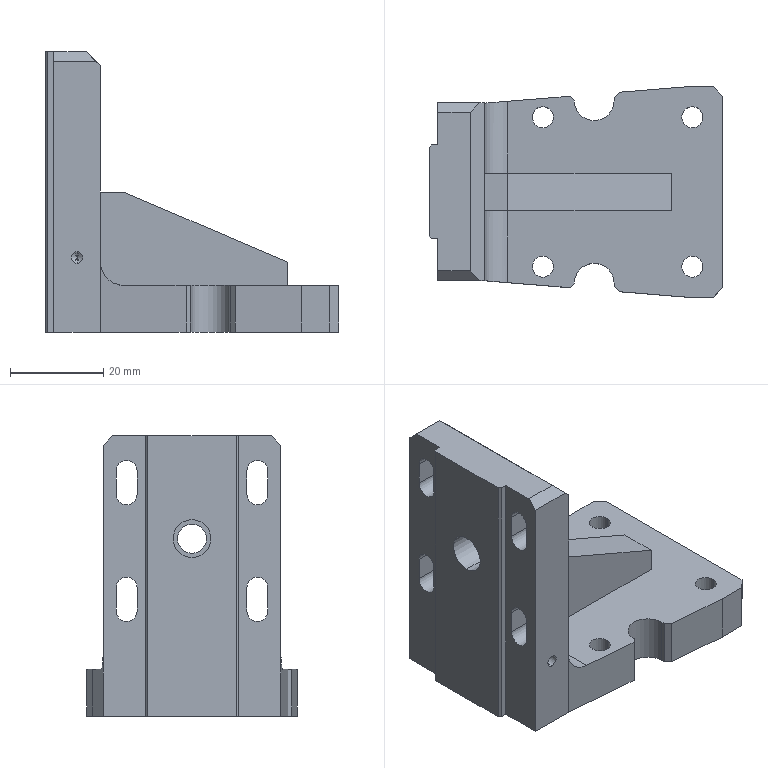Part | SolidWorks | features ICE 9, Chamfer 4, Cut 2, Extrusion 1, Fillet 1, HoleWzd 1, LPattern 1, MirrorPattern 1 | 1 solid | 88 faces | box 62.8 x 45 x 60 mm | volume 46658 mm3 | plane 51 | cylinder 33 | cone 4 | commonest cylinder face diameters 4.5 x16 6 x5 2.5 x4 6.2 x2 8.1 x2 8.5 x2